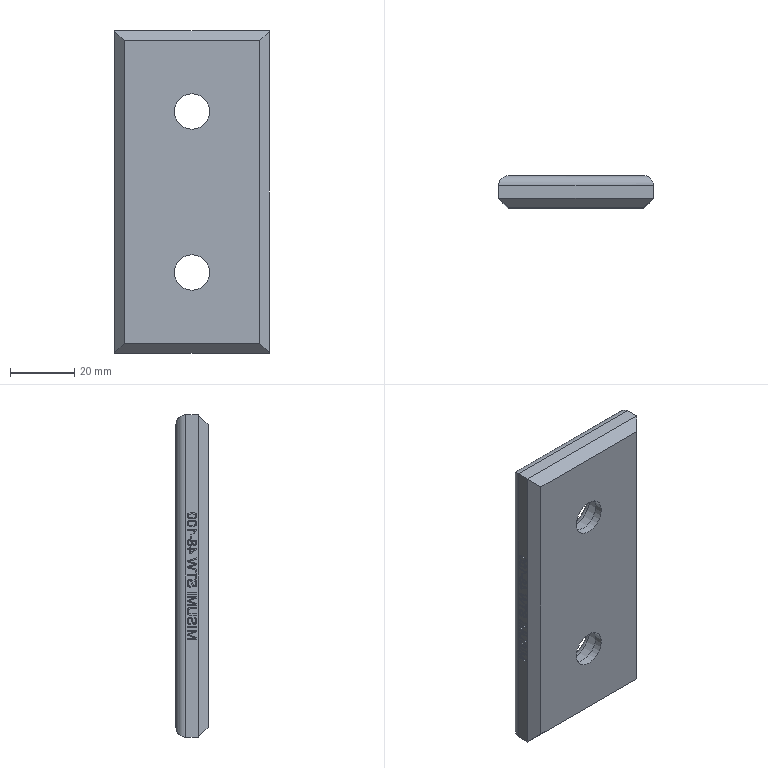Part | NX | features solid 2 | 1 solid | 154 faces | box 48 x 10 x 100 mm | volume 41954 mm3 | plane 107 | spline 37 | cylinder 8 | torus 2 | commonest cylinder face diameters 6 x4 11 x2 17.5 x2